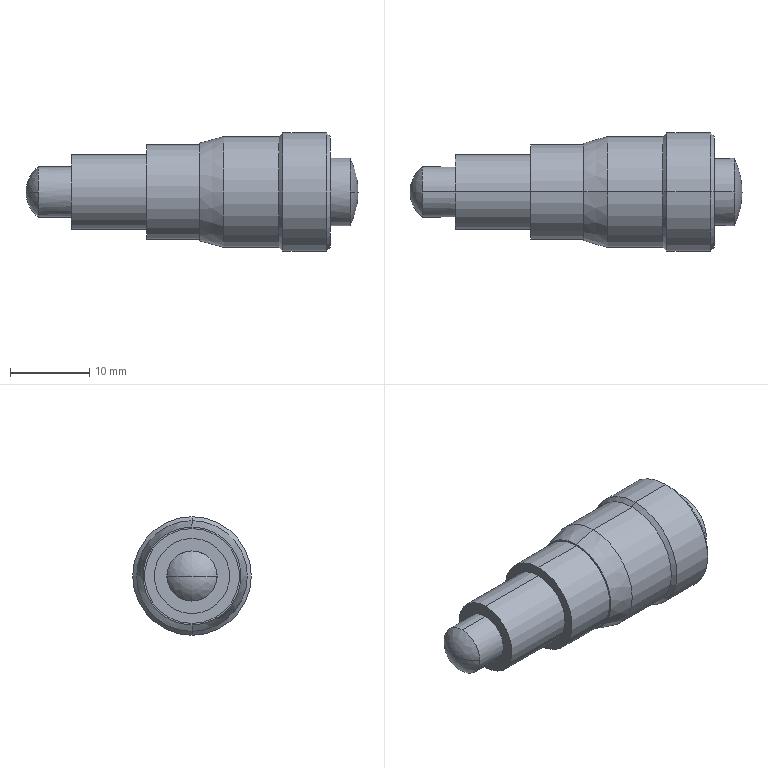Part | SolidWorks | features BaseBody 1 | 1 solid | 26 faces | box 42 x 15 x 15 mm | volume 4392 mm3 | cylinder 12 | cone 6 | spline 4 | plane 4 | commonest cylinder face diameters 6.35 x2 8.5 x2 9.5 x2 12 x2 14 x2 15 x2
STEP:
#1=CARTESIAN_POINT('',(26.75,0.,0.));
#2=VERTEX_POINT('',#1);
#3=CARTESIAN_POINT('',(25.746,4.25,0.));
#4=VERTEX_POINT('',#3);
#5=CARTESIAN_POINT('',(17.25,0.,0.));
#6=DIRECTION('',(0.,0.,1.));
#7=DIRECTION('',(1.,0.,0.));
#8=AXIS2_PLACEMENT_3D('',#5,#6,#7);
#9=CIRCLE('',#8,9.5);
#10=EDGE_CURVE('',#2,#4,#9,.T.);
#11=ORIENTED_EDGE('',*,*,#10,.F.);
#12=CARTESIAN_POINT('',(25.746,-4.25,0.));
#13=VERTEX_POINT('',#12);
#14=CARTESIAN_POINT('',(17.25,0.,0.));
#15=DIRECTION('',(0.,0.,-1.));
#16=DIRECTION('',(1.,0.,0.));
#17=AXIS2_PLACEMENT_3D('',#14,#15,#16);
#18=CIRCLE('',#17,9.5);
#19=EDGE_CURVE('',#2,#13,#18,.T.);
#20=ORIENTED_EDGE('',*,*,#19,.T.);
#21=CARTESIAN_POINT('',(25.746,0.,-4.25));
#22=VERTEX_POINT('',#21);
#23=CARTESIAN_POINT('',(25.746,0.,0.));
#24=DIRECTION('',(-1.,0.,0.));
#25=DIRECTION('',(0.,0.,-1.));
#26=AXIS2_PLACEMENT_3D('',#23,#24,#25);
#27=CIRCLE('',#26,4.25);
#28=EDGE_CURVE('',#22,#13,#27,.T.);
#29=ORIENTED_EDGE('',*,*,#28,.F.);
#30=CARTESIAN_POINT('',(25.746,0.,0.));
#31=DIRECTION('',(-1.,0.,0.));
#32=DIRECTION('',(0.,0.,-1.));
#33=AXIS2_PLACEMENT_3D('',#30,#31,#32);
#34=CIRCLE('',#33,4.25);
#35=EDGE_CURVE('',#4,#22,#34,.T.);
#36=ORIENTED_EDGE('',*,*,#35,.F.);
#37=EDGE_LOOP('',(#11,#20,#29,#36));
#38=FACE_OUTER_BOUND('',#37,.T.);
#39=CARTESIAN_POINT('',(26.75,0.,0.));
#40=CARTESIAN_POINT('',(26.75,0.,0.));
#41=CARTESIAN_POINT('',(26.75,0.,0.));
#42=CARTESIAN_POINT('',(26.75,0.,0.));
#43=CARTESIAN_POINT('',(26.75,-1.482,0.));
#44=CARTESIAN_POINT('',(26.75,-1.482,-2.964));
#45=CARTESIAN_POINT('',(26.75,1.482,-2.964));
#46=CARTESIAN_POINT('',(26.75,1.482,0.));
#47=CARTESIAN_POINT('',(26.409,-2.924,0.));
#48=CARTESIAN_POINT('',(26.409,-2.924,-5.849));
#49=CARTESIAN_POINT('',(26.409,2.924,-5.849));
#50=CARTESIAN_POINT('',(26.409,2.924,0.));
#51=CARTESIAN_POINT('',(25.746,-4.25,0.));
#52=CARTESIAN_POINT('',(25.746,-4.25,-8.5));
#53=CARTESIAN_POINT('',(25.746,4.25,-8.5));
#54=CARTESIAN_POINT('',(25.746,4.25,0.));
#55=(BOUNDED_SURFACE()B_SPLINE_SURFACE(3,3,((#39,#40,#41,#42),(#43,#44,#45,#46),(#47,#48,#49,#50),(#51,#52,#53,#54)),.UNSPECIFIED.,.F.,.F.,.T.)B_SPLINE_SURFACE_WITH_KNOTS((4,4),(4,4),(0.,1.),(0.,1.),.UNSPECIFIED.)GEOMETRIC_REPRESENTATION_ITEM()RATIONAL_B_SPLINE_SURFACE(((1.,0.3333,0.3333,1.),(0.9822,0.3274,0.3274,0.9822),(0.9822,0.3274,0.3274,0.9822),(1.,0.3333,0.3333,1.)))REPRESENTATION_ITEM('')SURFACE());
#56=ADVANCED_FACE('',(#38),#55,.T.);
#57=CARTESIAN_POINT('',(-13.683,-3.175,0.));
#58=VERTEX_POINT('',#57);
#59=CARTESIAN_POINT('',(-13.683,0.,-3.175));
#60=VERTEX_POINT('',#59);
#61=CARTESIAN_POINT('',(-13.683,0.,0.));
#62=DIRECTION('',(1.,0.,0.));
#63=DIRECTION('',(0.,0.,-1.));
#64=AXIS2_PLACEMENT_3D('',#61,#62,#63);
#65=CIRCLE('',#64,3.175);
#66=EDGE_CURVE('',#58,#60,#65,.T.);
#67=ORIENTED_EDGE('',*,*,#66,.F.);
#68=CARTESIAN_POINT('',(-15.25,0.,0.));
#69=VERTEX_POINT('',#68);
#70=CARTESIAN_POINT('',(-11.25,0.,0.));
#71=DIRECTION('',(0.,0.,-1.));
#72=DIRECTION('',(1.,0.,0.));
#73=AXIS2_PLACEMENT_3D('',#70,#71,#72);
#74=CIRCLE('',#73,4.);
#75=EDGE_CURVE('',#58,#69,#74,.T.);
#76=ORIENTED_EDGE('',*,*,#75,.T.);
#77=CARTESIAN_POINT('',(-13.683,3.175,0.));
#78=VERTEX_POINT('',#77);
#79=CARTESIAN_POINT('',(-11.25,0.,0.));
#80=DIRECTION('',(0.,0.,1.));
#81=DIRECTION('',(1.,0.,0.));
#82=AXIS2_PLACEMENT_3D('',#79,#80,#81);
#83=CIRCLE('',#82,4.);
#84=EDGE_CURVE('',#78,#69,#83,.T.);
#85=ORIENTED_EDGE('',*,*,#84,.F.);
#86=CARTESIAN_POINT('',(-13.683,0.,0.));
#87=DIRECTION('',(1.,0.,0.));
#88=DIRECTION('',(0.,0.,-1.));
#89=AXIS2_PLACEMENT_3D('',#86,#87,#88);
#90=CIRCLE('',#89,3.175);
#91=EDGE_CURVE('',#60,#78,#90,.T.);
#92=ORIENTED_EDGE('',*,*,#91,.F.);
#93=EDGE_LOOP('',(#67,#76,#85,#92));
#94=FACE_OUTER_BOUND('',#93,.T.);
#95=CARTESIAN_POINT('',(-13.683,-3.175,0.));
#96=CARTESIAN_POINT('',(-13.683,-3.175,-6.35));
#97=CARTESIAN_POINT('',(-13.683,3.175,-6.35));
#98=CARTESIAN_POINT('',(-13.683,3.175,0.));
#99=CARTESIAN_POINT('',(-14.689,-2.404,0.));
#100=CARTESIAN_POINT('',(-14.689,-2.404,-4.808));
#101=CARTESIAN_POINT('',(-14.689,2.404,-4.808));
#102=CARTESIAN_POINT('',(-14.689,2.404,0.));
#103=CARTESIAN_POINT('',(-15.25,-1.267,0.));
#104=CARTESIAN_POINT('',(-15.25,-1.267,-2.535));
#105=CARTESIAN_POINT('',(-15.25,1.267,-2.535));
#106=CARTESIAN_POINT('',(-15.25,1.267,0.));
#107=CARTESIAN_POINT('',(-15.25,0.,0.));
#108=CARTESIAN_POINT('',(-15.25,0.,0.));
#109=CARTESIAN_POINT('',(-15.25,0.,0.));
#110=CARTESIAN_POINT('',(-15.25,0.,0.));
#111=(BOUNDED_SURFACE()B_SPLINE_SURFACE(3,3,((#95,#96,#97,#98),(#99,#100,#101,#102),(#103,#104,#105,#106),(#107,#108,#109,#110)),.UNSPECIFIED.,.F.,.F.,.F.)B_SPLINE_SURFACE_WITH_KNOTS((4,4),(4,4),(0.,1.),(0.,1.),.UNSPECIFIED.)GEOMETRIC_REPRESENTATION_ITEM()RATIONAL_B_SPLINE_SURFACE(((1.,0.3333,0.3333,1.),(0.9312,0.3104,0.3104,0.9312),(0.9312,0.3104,0.3104,0.9312),(1.,0.3333,0.3333,1.)))REPRESENTATION_ITEM('')SURFACE());
#112=ADVANCED_FACE('',(#94),#111,.T.);
#113=CARTESIAN_POINT('',(9.75,0.,-7.));
#114=VERTEX_POINT('',#113);
#115=CARTESIAN_POINT('',(9.75,0.,7.));
#116=VERTEX_POINT('',#115);
#117=CARTESIAN_POINT('',(9.75,0.,0.));
#118=DIRECTION('',(1.,0.,0.));
#119=DIRECTION('',(0.,0.,-1.));
#120=AXIS2_PLACEMENT_3D('',#117,#118,#119);
#121=CIRCLE('',#120,7.);
#122=EDGE_CURVE('',#114,#116,#121,.T.);
#123=ORIENTED_EDGE('',*,*,#122,.T.);
#124=CARTESIAN_POINT('',(16.75,0.,7.));
#125=VERTEX_POINT('',#124);
#126=CARTESIAN_POINT('',(13.25,0.,7.));
#127=DIRECTION('',(1.,0.,0.));
#128=VECTOR('',#127,1000.);
#129=LINE('',#126,#128);
#130=EDGE_CURVE('',#116,#125,#129,.T.);
#131=ORIENTED_EDGE('',*,*,#130,.T.);
#132=CARTESIAN_POINT('',(16.75,0.,-7.));
#133=VERTEX_POINT('',#132);
#134=CARTESIAN_POINT('',(16.75,0.,0.));
#135=DIRECTION('',(-1.,0.,0.));
#136=DIRECTION('',(0.,0.,-1.));
#137=AXIS2_PLACEMENT_3D('',#134,#135,#136);
#138=CIRCLE('',#137,7.);
#139=EDGE_CURVE('',#125,#133,#138,.T.);
#140=ORIENTED_EDGE('',*,*,#139,.T.);
#141=CARTESIAN_POINT('',(13.25,0.,-7.));
#142=DIRECTION('',(1.,0.,0.));
#143=VECTOR('',#142,1000.);
#144=LINE('',#141,#143);
#145=EDGE_CURVE('',#114,#133,#144,.T.);
#146=ORIENTED_EDGE('',*,*,#145,.F.);
#147=EDGE_LOOP('',(#123,#131,#140,#146));
#148=FACE_OUTER_BOUND('',#147,.T.);
#149=CARTESIAN_POINT('',(13.25,0.,0.));
#150=DIRECTION('',(1.,0.,0.));
#151=DIRECTION('',(0.,0.,-1.));
#152=AXIS2_PLACEMENT_3D('',#149,#150,#151);
#153=CYLINDRICAL_SURFACE('',#152,7.);
#154=ADVANCED_FACE('',(#148),#153,.T.);
#155=CARTESIAN_POINT('',(6.75,0.,-6.196));
#156=VERTEX_POINT('',#155);
#157=CARTESIAN_POINT('',(6.75,0.,6.196));
#158=VERTEX_POINT('',#157);
#159=CARTESIAN_POINT('',(6.75,0.,0.));
#160=DIRECTION('',(1.,0.,0.));
#161=DIRECTION('',(0.,0.,-1.));
#162=AXIS2_PLACEMENT_3D('',#159,#160,#161);
#163=CIRCLE('',#162,6.196);
#164=EDGE_CURVE('',#156,#158,#163,.T.);
#165=ORIENTED_EDGE('',*,*,#164,.T.);
#166=CARTESIAN_POINT('',(9.75,0.,7.));
#167=DIRECTION('',(0.9659,0.,0.2588));
#168=VECTOR('',#167,1000.);
#169=LINE('',#166,#168);
#170=EDGE_CURVE('',#158,#116,#169,.T.);
#171=ORIENTED_EDGE('',*,*,#170,.T.);
#172=ORIENTED_EDGE('',*,*,#122,.F.);
#173=CARTESIAN_POINT('',(9.75,0.,-7.));
#174=DIRECTION('',(0.9659,0.,-0.2588));
#175=VECTOR('',#174,1000.);
#176=LINE('',#173,#175);
#177=EDGE_CURVE('',#156,#114,#176,.T.);
#178=ORIENTED_EDGE('',*,*,#177,.F.);
#179=EDGE_LOOP('',(#165,#171,#172,#178));
#180=FACE_OUTER_BOUND('',#179,.T.);
#181=CARTESIAN_POINT('',(9.75,0.,0.));
#182=DIRECTION('',(1.,0.,0.));
#183=DIRECTION('',(0.,0.,-1.));
#184=AXIS2_PLACEMENT_3D('',#181,#182,#183);
#185=CONICAL_SURFACE('',#184,7.,0.2618);
#186=ADVANCED_FACE('',(#180),#185,.T.);
#187=ORIENTED_EDGE('',*,*,#139,.F.);
#188=CARTESIAN_POINT('',(17.25,0.,7.5));
#189=VERTEX_POINT('',#188);
#190=CARTESIAN_POINT('',(17.25,0.,7.5));
#191=DIRECTION('',(0.7071,0.,0.7071));
#192=VECTOR('',#191,1000.);
#193=LINE('',#190,#192);
#194=EDGE_CURVE('',#125,#189,#193,.T.);
#195=ORIENTED_EDGE('',*,*,#194,.T.);
#196=CARTESIAN_POINT('',(17.25,0.,-7.5));
#197=VERTEX_POINT('',#196);
#198=CARTESIAN_POINT('',(17.25,0.,0.));
#199=DIRECTION('',(-1.,0.,0.));
#200=DIRECTION('',(0.,1.,0.));
#201=AXIS2_PLACEMENT_3D('',#198,#199,#200);
#202=CIRCLE('',#201,7.5);
#203=EDGE_CURVE('',#189,#197,#202,.T.);
#204=ORIENTED_EDGE('',*,*,#203,.T.);
#205=CARTESIAN_POINT('',(17.25,0.,-7.5));
#206=DIRECTION('',(0.7071,0.,-0.7071));
#207=VECTOR('',#206,1000.);
#208=LINE('',#205,#207);
#209=EDGE_CURVE('',#133,#197,#208,.T.);
#210=ORIENTED_EDGE('',*,*,#209,.F.);
#211=EDGE_LOOP('',(#187,#195,#204,#210));
#212=FACE_OUTER_BOUND('',#211,.T.);
#213=CARTESIAN_POINT('',(17.25,0.,0.));
#214=DIRECTION('',(1.,0.,0.));
#215=DIRECTION('',(0.,0.,-1.));
#216=AXIS2_PLACEMENT_3D('',#213,#214,#215);
#217=CONICAL_SURFACE('',#216,7.5,0.7854);
#218=ADVANCED_FACE('',(#212),#217,.T.);
#219=ORIENTED_EDGE('',*,*,#203,.F.);
#220=CARTESIAN_POINT('',(22.75,0.,7.5));
#221=VERTEX_POINT('',#220);
#222=CARTESIAN_POINT('',(20.,0.,7.5));
#223=DIRECTION('',(1.,0.,0.));
#224=VECTOR('',#223,1000.);
#225=LINE('',#222,#224);
#226=EDGE_CURVE('',#189,#221,#225,.T.);
#227=ORIENTED_EDGE('',*,*,#226,.T.);
#228=CARTESIAN_POINT('',(22.75,0.,-7.5));
#229=VERTEX_POINT('',#228);
#230=CARTESIAN_POINT('',(22.75,0.,0.));
#231=DIRECTION('',(-1.,0.,0.));
#232=DIRECTION('',(0.,0.,-1.));
#233=AXIS2_PLACEMENT_3D('',#230,#231,#232);
#234=CIRCLE('',#233,7.5);
#235=EDGE_CURVE('',#221,#229,#234,.T.);
#236=ORIENTED_EDGE('',*,*,#235,.T.);
#237=CARTESIAN_POINT('',(20.,0.,-7.5));
#238=DIRECTION('',(1.,0.,0.));
#239=VECTOR('',#238,1000.);
#240=LINE('',#237,#239);
#241=EDGE_CURVE('',#197,#229,#240,.T.);
#242=ORIENTED_EDGE('',*,*,#241,.F.);
#243=EDGE_LOOP('',(#219,#227,#236,#242));
#244=FACE_OUTER_BOUND('',#243,.T.);
#245=CARTESIAN_POINT('',(20.,0.,0.));
#246=DIRECTION('',(1.,0.,0.));
#247=DIRECTION('',(0.,0.,-1.));
#248=AXIS2_PLACEMENT_3D('',#245,#246,#247);
#249=CYLINDRICAL_SURFACE('',#248,7.5);
#250=ADVANCED_FACE('',(#244),#249,.T.);
#251=CARTESIAN_POINT('',(0.,0.,-6.));
#252=VERTEX_POINT('',#251);
#253=CARTESIAN_POINT('',(0.,0.,6.));
#254=VERTEX_POINT('',#253);
#255=CARTESIAN_POINT('',(0.,0.,0.));
#256=DIRECTION('',(1.,0.,0.));
#257=DIRECTION('',(0.,0.,-1.));
#258=AXIS2_PLACEMENT_3D('',#255,#256,#257);
#259=CIRCLE('',#258,6.);
#260=EDGE_CURVE('',#252,#254,#259,.T.);
#261=ORIENTED_EDGE('',*,*,#260,.T.);
#262=CARTESIAN_POINT('',(6.75,0.,6.));
#263=VERTEX_POINT('',#262);
#264=CARTESIAN_POINT('',(3.375,0.,6.));
#265=DIRECTION('',(1.,0.,0.));
#266=VECTOR('',#265,1000.);
#267=LINE('',#264,#266);
#268=EDGE_CURVE('',#254,#263,#267,.T.);
#269=ORIENTED_EDGE('',*,*,#268,.T.);
#270=CARTESIAN_POINT('',(6.75,0.,-6.));
#271=VERTEX_POINT('',#270);
#272=CARTESIAN_POINT('',(6.75,0.,0.));
#273=DIRECTION('',(1.,0.,0.));
#274=DIRECTION('',(0.,0.,-1.));
#275=AXIS2_PLACEMENT_3D('',#272,#273,#274);
#276=CIRCLE('',#275,6.);
#277=EDGE_CURVE('',#271,#263,#276,.T.);
#278=ORIENTED_EDGE('',*,*,#277,.F.);
#279=CARTESIAN_POINT('',(3.375,0.,-6.));
#280=DIRECTION('',(1.,0.,0.));
#281=VECTOR('',#280,1000.);
#282=LINE('',#279,#281);
#283=EDGE_CURVE('',#252,#271,#282,.T.);
#284=ORIENTED_EDGE('',*,*,#283,.F.);
#285=EDGE_LOOP('',(#261,#269,#278,#284));
#286=FACE_OUTER_BOUND('',#285,.T.);
#287=CARTESIAN_POINT('',(3.375,0.,0.));
#288=DIRECTION('',(1.,0.,0.));
#289=DIRECTION('',(0.,0.,-1.));
#290=AXIS2_PLACEMENT_3D('',#287,#288,#289);
#291=CYLINDRICAL_SURFACE('',#290,6.);
#292=ADVANCED_FACE('',(#286),#291,.T.);
#293=CARTESIAN_POINT('',(23.25,0.,7.));
#294=VERTEX_POINT('',#293);
#295=CARTESIAN_POINT('',(23.25,0.,-7.));
#296=VERTEX_POINT('',#295);
#297=CARTESIAN_POINT('',(23.25,0.,0.));
#298=DIRECTION('',(-1.,0.,0.));
#299=DIRECTION('',(0.,0.,1.));
#300=AXIS2_PLACEMENT_3D('',#297,#298,#299);
#301=CIRCLE('',#300,7.);
#302=EDGE_CURVE('',#294,#296,#301,.T.);
#303=ORIENTED_EDGE('',*,*,#302,.T.);
#304=CARTESIAN_POINT('',(22.75,0.,-7.5));
#305=DIRECTION('',(-0.7071,0.,-0.7071));
#306=VECTOR('',#305,1000.);
#307=LINE('',#304,#306);
#308=EDGE_CURVE('',#296,#229,#307,.T.);
#309=ORIENTED_EDGE('',*,*,#308,.T.);
#310=ORIENTED_EDGE('',*,*,#235,.F.);
#311=CARTESIAN_POINT('',(22.75,0.,7.5));
#312=DIRECTION('',(-0.7071,0.,0.7071));
#313=VECTOR('',#312,1000.);
#314=LINE('',#311,#313);
#315=EDGE_CURVE('',#294,#221,#314,.T.);
#316=ORIENTED_EDGE('',*,*,#315,.F.);
#317=EDGE_LOOP('',(#303,#309,#310,#316));
#318=FACE_OUTER_BOUND('',#317,.T.);
#319=CARTESIAN_POINT('',(22.75,0.,0.));
#320=DIRECTION('',(-1.,0.,0.));
#321=DIRECTION('',(0.,0.,1.));
#322=AXIS2_PLACEMENT_3D('',#319,#320,#321);
#323=CONICAL_SURFACE('',#322,7.5,0.7854);
#324=ADVANCED_FACE('',(#318),#323,.T.);
#325=CARTESIAN_POINT('',(-9.5,0.,-4.75));
#326=VERTEX_POINT('',#325);
#327=CARTESIAN_POINT('',(-9.5,0.,4.75));
#328=VERTEX_POINT('',#327);
#329=CARTESIAN_POINT('',(-9.5,0.,0.));
#330=DIRECTION('',(1.,0.,0.));
#331=DIRECTION('',(0.,0.,-1.));
#332=AXIS2_PLACEMENT_3D('',#329,#330,#331);
#333=CIRCLE('',#332,4.75);
#334=EDGE_CURVE('',#326,#328,#333,.T.);
#335=ORIENTED_EDGE('',*,*,#334,.T.);
#336=CARTESIAN_POINT('',(0.,0.,4.75));
#337=VERTEX_POINT('',#336);
#338=CARTESIAN_POINT('',(-4.75,0.,4.75));
#339=DIRECTION('',(1.,0.,0.));
#340=VECTOR('',#339,1000.);
#341=LINE('',#338,#340);
#342=EDGE_CURVE('',#328,#337,#341,.T.);
#343=ORIENTED_EDGE('',*,*,#342,.T.);
#344=CARTESIAN_POINT('',(0.,0.,-4.75));
#345=VERTEX_POINT('',#344);
#346=CARTESIAN_POINT('',(0.,0.,0.));
#347=DIRECTION('',(1.,0.,0.));
#348=DIRECTION('',(0.,0.,-1.));
#349=AXIS2_PLACEMENT_3D('',#346,#347,#348);
#350=CIRCLE('',#349,4.75);
#351=EDGE_CURVE('',#345,#337,#350,.T.);
#352=ORIENTED_EDGE('',*,*,#351,.F.);
#353=CARTESIAN_POINT('',(-4.75,0.,-4.75));
#354=DIRECTION('',(1.,0.,0.));
#355=VECTOR('',#354,1000.);
#356=LINE('',#353,#355);
#357=EDGE_CURVE('',#326,#345,#356,.T.);
#358=ORIENTED_EDGE('',*,*,#357,.F.);
#359=EDGE_LOOP('',(#335,#343,#352,#358));
#360=FACE_OUTER_BOUND('',#359,.T.);
#361=CARTESIAN_POINT('',(-4.75,0.,0.));
#362=DIRECTION('',(1.,0.,0.));
#363=DIRECTION('',(0.,0.,-1.));
#364=AXIS2_PLACEMENT_3D('',#361,#362,#363);
#365=CYLINDRICAL_SURFACE('',#364,4.75);
#366=ADVANCED_FACE('',(#360),#365,.T.);
#367=CARTESIAN_POINT('',(23.25,0.,4.25));
#368=VERTEX_POINT('',#367);
#369=CARTESIAN_POINT('',(23.25,0.,-4.25));
#370=VERTEX_POINT('',#369);
#371=CARTESIAN_POINT('',(23.25,0.,0.));
#372=DIRECTION('',(-1.,0.,0.));
#373=DIRECTION('',(0.,0.,-1.));
#374=AXIS2_PLACEMENT_3D('',#371,#372,#373);
#375=CIRCLE('',#374,4.25);
#376=EDGE_CURVE('',#368,#370,#375,.T.);
#377=ORIENTED_EDGE('',*,*,#376,.F.);
#378=CARTESIAN_POINT('',(25.746,0.,4.25));
#379=VERTEX_POINT('',#378);
#380=CARTESIAN_POINT('',(24.498,0.,4.25));
#381=DIRECTION('',(1.,0.,0.));
#382=VECTOR('',#381,1000.);
#383=LINE('',#380,#382);
#384=EDGE_CURVE('',#368,#379,#383,.T.);
#385=ORIENTED_EDGE('',*,*,#384,.T.);
#386=CARTESIAN_POINT('',(25.746,0.,0.));
#387=DIRECTION('',(-1.,0.,0.));
#388=DIRECTION('',(0.,0.,-1.));
#389=AXIS2_PLACEMENT_3D('',#386,#387,#388);
#390=CIRCLE('',#389,4.25);
#391=EDGE_CURVE('',#379,#4,#390,.T.);
#392=ORIENTED_EDGE('',*,*,#391,.T.);
#393=ORIENTED_EDGE('',*,*,#35,.T.);
#394=CARTESIAN_POINT('',(24.498,0.,-4.25));
#395=DIRECTION('',(1.,0.,0.));
#396=VECTOR('',#395,1000.);
#397=LINE('',#394,#396);
#398=EDGE_CURVE('',#370,#22,#397,.T.);
#399=ORIENTED_EDGE('',*,*,#398,.F.);
#400=EDGE_LOOP('',(#377,#385,#392,#393,#399));
#401=FACE_OUTER_BOUND('',#400,.T.);
#402=CARTESIAN_POINT('',(24.498,0.,0.));
#403=DIRECTION('',(1.,0.,0.));
#404=DIRECTION('',(0.,0.,-1.));
#405=AXIS2_PLACEMENT_3D('',#402,#403,#404);
#406=CYLINDRICAL_SURFACE('',#405,4.25);
#407=ADVANCED_FACE('',(#401),#406,.T.);
#408=ORIENTED_EDGE('',*,*,#91,.T.);
#409=CARTESIAN_POINT('',(-13.683,0.,3.175));
#410=VERTEX_POINT('',#409);
#411=CARTESIAN_POINT('',(-13.683,0.,0.));
#412=DIRECTION('',(1.,0.,0.));
#413=DIRECTION('',(0.,0.,-1.));
#414=AXIS2_PLACEMENT_3D('',#411,#412,#413);
#415=CIRCLE('',#414,3.175);
#416=EDGE_CURVE('',#78,#410,#415,.T.);
#417=ORIENTED_EDGE('',*,*,#416,.T.);
#418=CARTESIAN_POINT('',(-9.5,0.,3.175));
#419=VERTEX_POINT('',#418);
#420=CARTESIAN_POINT('',(-11.591,0.,3.175));
#421=DIRECTION('',(1.,0.,0.));
#422=VECTOR('',#421,1000.);
#423=LINE('',#420,#422);
#424=EDGE_CURVE('',#410,#419,#423,.T.);
#425=ORIENTED_EDGE('',*,*,#424,.T.);
#426=CARTESIAN_POINT('',(-9.5,0.,-3.175));
#427=VERTEX_POINT('',#426);
#428=CARTESIAN_POINT('',(-9.5,0.,0.));
#429=DIRECTION('',(1.,0.,0.));
#430=DIRECTION('',(0.,0.,-1.));
#431=AXIS2_PLACEMENT_3D('',#428,#429,#430);
#432=CIRCLE('',#431,3.175);
#433=EDGE_CURVE('',#427,#419,#432,.T.);
#434=ORIENTED_EDGE('',*,*,#433,.F.);
#435=CARTESIAN_POINT('',(-11.591,0.,-3.175));
#436=DIRECTION('',(1.,0.,0.));
#437=VECTOR('',#436,1000.);
#438=LINE('',#435,#437);
#439=EDGE_CURVE('',#60,#427,#438,.T.);
#440=ORIENTED_EDGE('',*,*,#439,.F.);
#441=EDGE_LOOP('',(#408,#417,#425,#434,#440));
#442=FACE_OUTER_BOUND('',#441,.T.);
#443=CARTESIAN_POINT('',(-11.591,0.,0.));
#444=DIRECTION('',(1.,0.,0.));
#445=DIRECTION('',(0.,0.,-1.));
#446=AXIS2_PLACEMENT_3D('',#443,#444,#445);
#447=CYLINDRICAL_SURFACE('',#446,3.175);
#448=ADVANCED_FACE('',(#442),#447,.T.);
#449=ORIENTED_EDGE('',*,*,#130,.F.);
#450=CARTESIAN_POINT('',(9.75,0.,0.));
#451=DIRECTION('',(1.,0.,0.));
#452=DIRECTION('',(0.,0.,-1.));
#453=AXIS2_PLACEMENT_3D('',#450,#451,#452);
#454=CIRCLE('',#453,7.);
#455=EDGE_CURVE('',#116,#114,#454,.T.);
#456=ORIENTED_EDGE('',*,*,#455,.T.);
#457=ORIENTED_EDGE('',*,*,#145,.T.);
#458=CARTESIAN_POINT('',(16.75,0.,0.));
#459=DIRECTION('',(-1.,0.,0.));
#460=DIRECTION('',(0.,0.,-1.));
#461=AXIS2_PLACEMENT_3D('',#458,#459,#460);
#462=CIRCLE('',#461,7.);
#463=EDGE_CURVE('',#133,#125,#462,.T.);
#464=ORIENTED_EDGE('',*,*,#463,.T.);
#465=EDGE_LOOP('',(#449,#456,#457,#464));
#466=FACE_OUTER_BOUND('',#465,.T.);
#467=CARTESIAN_POINT('',(13.25,0.,0.));
#468=DIRECTION('',(1.,0.,0.));
#469=DIRECTION('',(0.,0.,-1.));
#470=AXIS2_PLACEMENT_3D('',#467,#468,#469);
#471=CYLINDRICAL_SURFACE('',#470,7.);
#472=ADVANCED_FACE('',(#466),#471,.T.);
#473=ORIENTED_EDGE('',*,*,#170,.F.);
#474=CARTESIAN_POINT('',(6.75,0.,0.));
#475=DIRECTION('',(1.,0.,0.));
#476=DIRECTION('',(0.,0.,-1.));
#477=AXIS2_PLACEMENT_3D('',#474,#475,#476);
#478=CIRCLE('',#477,6.196);
#479=EDGE_CURVE('',#158,#156,#478,.T.);
#480=ORIENTED_EDGE('',*,*,#479,.T.);
#481=ORIENTED_EDGE('',*,*,#177,.T.);
#482=ORIENTED_EDGE('',*,*,#455,.F.);
#483=EDGE_LOOP('',(#473,#480,#481,#482));
#484=FACE_OUTER_BOUND('',#483,.T.);
#485=CARTESIAN_POINT('',(9.75,0.,0.));
#486=DIRECTION('',(1.,0.,0.));
#487=DIRECTION('',(0.,0.,-1.));
#488=AXIS2_PLACEMENT_3D('',#485,#486,#487);
#489=CONICAL_SURFACE('',#488,7.,0.2618);
#490=ADVANCED_FACE('',(#484),#489,.T.);
#491=ORIENTED_EDGE('',*,*,#194,.F.);
#492=ORIENTED_EDGE('',*,*,#463,.F.);
#493=ORIENTED_EDGE('',*,*,#209,.T.);
#494=CARTESIAN_POINT('',(17.25,0.,0.));
#495=DIRECTION('',(-1.,0.,0.));
#496=DIRECTION('',(0.,1.,0.));
#497=AXIS2_PLACEMENT_3D('',#494,#495,#496);
#498=CIRCLE('',#497,7.5);
#499=EDGE_CURVE('',#197,#189,#498,.T.);
#500=ORIENTED_EDGE('',*,*,#499,.T.);
#501=EDGE_LOOP('',(#491,#492,#493,#500));
#502=FACE_OUTER_BOUND('',#501,.T.);
#503=CARTESIAN_POINT('',(17.25,0.,0.));
#504=DIRECTION('',(1.,0.,0.));
#505=DIRECTION('',(0.,0.,-1.));
#506=AXIS2_PLACEMENT_3D('',#503,#504,#505);
#507=CONICAL_SURFACE('',#506,7.5,0.7854);
#508=ADVANCED_FACE('',(#502),#507,.T.);
#509=ORIENTED_EDGE('',*,*,#164,.F.);
#510=ORIENTED_EDGE('',*,*,#479,.F.);
#511=EDGE_LOOP('',(#509,#510));
#512=FACE_OUTER_BOUND('',#511,.T.);
#513=ORIENTED_EDGE('',*,*,#277,.T.);
#514=CARTESIAN_POINT('',(6.75,0.,0.));
#515=DIRECTION('',(1.,0.,0.));
#516=DIRECTION('',(0.,0.,-1.));
#517=AXIS2_PLACEMENT_3D('',#514,#515,#516);
#518=CIRCLE('',#517,6.);
#519=EDGE_CURVE('',#263,#271,#518,.T.);
#520=ORIENTED_EDGE('',*,*,#519,.T.);
#521=EDGE_LOOP('',(#513,#520));
#522=FACE_BOUND('',#521,.T.);
#523=CARTESIAN_POINT('',(6.75,6.098,0.));
#524=DIRECTION('',(-1.,0.,0.));
#525=DIRECTION('',(0.,0.,1.));
#526=AXIS2_PLACEMENT_3D('',#523,#524,#525);
#527=PLANE('',#526);
#528=ADVANCED_FACE('',(#512,#522),#527,.T.);
#529=ORIENTED_EDGE('',*,*,#226,.F.);
#530=ORIENTED_EDGE('',*,*,#499,.F.);
#531=ORIENTED_EDGE('',*,*,#241,.T.);
#532=CARTESIAN_POINT('',(22.75,0.,0.));
#533=DIRECTION('',(-1.,0.,0.));
#534=DIRECTION('',(0.,0.,-1.));
#535=AXIS2_PLACEMENT_3D('',#532,#533,#534);
#536=CIRCLE('',#535,7.5);
#537=EDGE_CURVE('',#229,#221,#536,.T.);
#538=ORIENTED_EDGE('',*,*,#537,.T.);
#539=EDGE_LOOP('',(#529,#530,#531,#538));
#540=FACE_OUTER_BOUND('',#539,.T.);
#541=CARTESIAN_POINT('',(20.,0.,0.));
#542=DIRECTION('',(1.,0.,0.));
#543=DIRECTION('',(0.,0.,-1.));
#544=AXIS2_PLACEMENT_3D('',#541,#542,#543);
#545=CYLINDRICAL_SURFACE('',#544,7.5);
#546=ADVANCED_FACE('',(#540),#545,.T.);
#547=ORIENTED_EDGE('',*,*,#268,.F.);
#548=CARTESIAN_POINT('',(0.,0.,0.));
#549=DIRECTION('',(1.,0.,0.));
#550=DIRECTION('',(0.,0.,-1.));
#551=AXIS2_PLACEMENT_3D('',#548,#549,#550);
#552=CIRCLE('',#551,6.);
#553=EDGE_CURVE('',#254,#252,#552,.T.);
#554=ORIENTED_EDGE('',*,*,#553,.T.);
#555=ORIENTED_EDGE('',*,*,#283,.T.);
#556=ORIENTED_EDGE('',*,*,#519,.F.);
#557=EDGE_LOOP('',(#547,#554,#555,#556));
#558=FACE_OUTER_BOUND('',#557,.T.);
#559=CARTESIAN_POINT('',(3.375,0.,0.));
#560=DIRECTION('',(1.,0.,0.));
#561=DIRECTION('',(0.,0.,-1.));
#562=AXIS2_PLACEMENT_3D('',#559,#560,#561);
#563=CYLINDRICAL_SURFACE('',#562,6.);
#564=ADVANCED_FACE('',(#558),#563,.T.);
#565=ORIENTED_EDGE('',*,*,#308,.F.);
#566=CARTESIAN_POINT('',(23.25,0.,0.));
#567=DIRECTION('',(-1.,0.,0.));
#568=DIRECTION('',(0.,0.,1.));
#569=AXIS2_PLACEMENT_3D('',#566,#567,#568);
#570=CIRCLE('',#569,7.);
#571=EDGE_CURVE('',#296,#294,#570,.T.);
#572=ORIENTED_EDGE('',*,*,#571,.T.);
#573=ORIENTED_EDGE('',*,*,#315,.T.);
#574=ORIENTED_EDGE('',*,*,#537,.F.);
#575=EDGE_LOOP('',(#565,#572,#573,#574));
#576=FACE_OUTER_BOUND('',#575,.T.);
#577=CARTESIAN_POINT('',(22.75,0.,0.));
#578=DIRECTION('',(-1.,0.,0.));
#579=DIRECTION('',(0.,0.,1.));
#580=AXIS2_PLACEMENT_3D('',#577,#578,#579);
#581=CONICAL_SURFACE('',#580,7.5,0.7854);
#582=ADVANCED_FACE('',(#576),#581,.T.);
#583=ORIENTED_EDGE('',*,*,#260,.F.);
#584=ORIENTED_EDGE('',*,*,#553,.F.);
#585=EDGE_LOOP('',(#583,#584));
#586=FACE_OUTER_BOUND('',#585,.T.);
#587=ORIENTED_EDGE('',*,*,#351,.T.);
#588=CARTESIAN_POINT('',(0.,0.,0.));
#589=DIRECTION('',(1.,0.,0.));
#590=DIRECTION('',(0.,0.,-1.));
#591=AXIS2_PLACEMENT_3D('',#588,#589,#590);
#592=CIRCLE('',#591,4.75);
#593=EDGE_CURVE('',#337,#345,#592,.T.);
#594=ORIENTED_EDGE('',*,*,#593,.T.);
#595=EDGE_LOOP('',(#587,#594));
#596=FACE_BOUND('',#595,.T.);
#597=CARTESIAN_POINT('',(0.,5.375,0.));
#598=DIRECTION('',(-1.,0.,0.));
#599=DIRECTION('',(0.,0.,1.));
#600=AXIS2_PLACEMENT_3D('',#597,#598,#599);
#601=PLANE('',#600);
#602=ADVANCED_FACE('',(#586,#596),#601,.T.);
#603=CARTESIAN_POINT('',(23.25,0.,0.));
#604=DIRECTION('',(-1.,0.,0.));
#605=DIRECTION('',(0.,0.,-1.));
#606=AXIS2_PLACEMENT_3D('',#603,#604,#605);
#607=CIRCLE('',#606,4.25);
#608=EDGE_CURVE('',#370,#368,#607,.T.);
#609=ORIENTED_EDGE('',*,*,#608,.T.);
#610=ORIENTED_EDGE('',*,*,#376,.T.);
#611=EDGE_LOOP('',(#609,#610));
#612=FACE_BOUND('',#611,.T.);
#613=ORIENTED_EDGE('',*,*,#302,.F.);
#614=ORIENTED_EDGE('',*,*,#571,.F.);
#615=EDGE_LOOP('',(#613,#614));
#616=FACE_OUTER_BOUND('',#615,.T.);
#617=CARTESIAN_POINT('',(23.25,5.625,0.));
#618=DIRECTION('',(1.,0.,0.));
#619=DIRECTION('',(0.,0.,-1.));
#620=AXIS2_PLACEMENT_3D('',#617,#618,#619);
#621=PLANE('',#620);
#622=ADVANCED_FACE('',(#612,#616),#621,.T.);
#623=ORIENTED_EDGE('',*,*,#342,.F.);
#624=CARTESIAN_POINT('',(-9.5,0.,0.));
#625=DIRECTION('',(1.,0.,0.));
#626=DIRECTION('',(0.,0.,-1.));
#627=AXIS2_PLACEMENT_3D('',#624,#625,#626);
#628=CIRCLE('',#627,4.75);
#629=EDGE_CURVE('',#328,#326,#628,.T.);
#630=ORIENTED_EDGE('',*,*,#629,.T.);
#631=ORIENTED_EDGE('',*,*,#357,.T.);
#632=ORIENTED_EDGE('',*,*,#593,.F.);
#633=EDGE_LOOP('',(#623,#630,#631,#632));
#634=FACE_OUTER_BOUND('',#633,.T.);
#635=CARTESIAN_POINT('',(-4.75,0.,0.));
#636=DIRECTION('',(1.,0.,0.));
#637=DIRECTION('',(0.,0.,-1.));
#638=AXIS2_PLACEMENT_3D('',#635,#636,#637);
#639=CYLINDRICAL_SURFACE('',#638,4.75);
#640=ADVANCED_FACE('',(#634),#639,.T.);
#641=ORIENTED_EDGE('',*,*,#384,.F.);
#642=ORIENTED_EDGE('',*,*,#608,.F.);
#643=ORIENTED_EDGE('',*,*,#398,.T.);
#644=ORIENTED_EDGE('',*,*,#28,.T.);
#645=CARTESIAN_POINT('',(25.746,0.,0.));
#646=DIRECTION('',(-1.,0.,0.));
#647=DIRECTION('',(0.,0.,-1.));
#648=AXIS2_PLACEMENT_3D('',#645,#646,#647);
#649=CIRCLE('',#648,4.25);
#650=EDGE_CURVE('',#13,#379,#649,.T.);
#651=ORIENTED_EDGE('',*,*,#650,.T.);
#652=EDGE_LOOP('',(#641,#642,#643,#644,#651));
#653=FACE_OUTER_BOUND('',#652,.T.);
#654=CARTESIAN_POINT('',(24.498,0.,0.));
#655=DIRECTION('',(1.,0.,0.));
#656=DIRECTION('',(0.,0.,-1.));
#657=AXIS2_PLACEMENT_3D('',#654,#655,#656);
#658=CYLINDRICAL_SURFACE('',#657,4.25);
#659=ADVANCED_FACE('',(#653),#658,.T.);
#660=ORIENTED_EDGE('',*,*,#334,.F.);
#661=ORIENTED_EDGE('',*,*,#629,.F.);
#662=EDGE_LOOP('',(#660,#661));
#663=FACE_OUTER_BOUND('',#662,.T.);
#664=ORIENTED_EDGE('',*,*,#433,.T.);
#665=CARTESIAN_POINT('',(-9.5,0.,0.));
#666=DIRECTION('',(1.,0.,0.));
#667=DIRECTION('',(0.,0.,-1.));
#668=AXIS2_PLACEMENT_3D('',#665,#666,#667);
#669=CIRCLE('',#668,3.175);
#670=EDGE_CURVE('',#419,#427,#669,.T.);
#671=ORIENTED_EDGE('',*,*,#670,.T.);
#672=EDGE_LOOP('',(#664,#671));
#673=FACE_BOUND('',#672,.T.);
#674=CARTESIAN_POINT('',(-9.5,3.962,0.));
#675=DIRECTION('',(-1.,0.,0.));
#676=DIRECTION('',(0.,0.,1.));
#677=AXIS2_PLACEMENT_3D('',#674,#675,#676);
#678=PLANE('',#677);
#679=ADVANCED_FACE('',(#663,#673),#678,.T.);
#680=ORIENTED_EDGE('',*,*,#19,.F.);
#681=ORIENTED_EDGE('',*,*,#10,.T.);
#682=ORIENTED_EDGE('',*,*,#391,.F.);
#683=ORIENTED_EDGE('',*,*,#650,.F.);
#684=EDGE_LOOP('',(#680,#681,#682,#683));
#685=FACE_OUTER_BOUND('',#684,.T.);
#686=CARTESIAN_POINT('',(26.75,0.,0.));
#687=CARTESIAN_POINT('',(26.75,0.,0.));
#688=CARTESIAN_POINT('',(26.75,0.,0.));
#689=CARTESIAN_POINT('',(26.75,0.,0.));
#690=CARTESIAN_POINT('',(26.75,1.482,0.));
#691=CARTESIAN_POINT('',(26.75,1.482,2.964));
#692=CARTESIAN_POINT('',(26.75,-1.482,2.964));
#693=CARTESIAN_POINT('',(26.75,-1.482,0.));
#694=CARTESIAN_POINT('',(26.409,2.924,0.));
#695=CARTESIAN_POINT('',(26.409,2.924,5.849));
#696=CARTESIAN_POINT('',(26.409,-2.924,5.849));
#697=CARTESIAN_POINT('',(26.409,-2.924,0.));
#698=CARTESIAN_POINT('',(25.746,4.25,0.));
#699=CARTESIAN_POINT('',(25.746,4.25,8.5));
#700=CARTESIAN_POINT('',(25.746,-4.25,8.5));
#701=CARTESIAN_POINT('',(25.746,-4.25,0.));
#702=(BOUNDED_SURFACE()B_SPLINE_SURFACE(3,3,((#686,#687,#688,#689),(#690,#691,#692,#693),(#694,#695,#696,#697),(#698,#699,#700,#701)),.UNSPECIFIED.,.F.,.F.,.T.)B_SPLINE_SURFACE_WITH_KNOTS((4,4),(4,4),(0.,1.),(0.,1.),.UNSPECIFIED.)GEOMETRIC_REPRESENTATION_ITEM()RATIONAL_B_SPLINE_SURFACE(((1.,0.3333,0.3333,1.),(0.9822,0.3274,0.3274,0.9822),(0.9822,0.3274,0.3274,0.9822),(1.,0.3333,0.3333,1.)))REPRESENTATION_ITEM('')SURFACE());
#703=ADVANCED_FACE('',(#685),#702,.T.);
#704=ORIENTED_EDGE('',*,*,#424,.F.);
#705=CARTESIAN_POINT('',(-13.683,0.,0.));
#706=DIRECTION('',(1.,0.,0.));
#707=DIRECTION('',(0.,0.,-1.));
#708=AXIS2_PLACEMENT_3D('',#705,#706,#707);
#709=CIRCLE('',#708,3.175);
#710=EDGE_CURVE('',#410,#58,#709,.T.);
#711=ORIENTED_EDGE('',*,*,#710,.T.);
#712=ORIENTED_EDGE('',*,*,#66,.T.);
#713=ORIENTED_EDGE('',*,*,#439,.T.);
#714=ORIENTED_EDGE('',*,*,#670,.F.);
#715=EDGE_LOOP('',(#704,#711,#712,#713,#714));
#716=FACE_OUTER_BOUND('',#715,.T.);
#717=CARTESIAN_POINT('',(-11.591,0.,0.));
#718=DIRECTION('',(1.,0.,0.));
#719=DIRECTION('',(0.,0.,-1.));
#720=AXIS2_PLACEMENT_3D('',#717,#718,#719);
#721=CYLINDRICAL_SURFACE('',#720,3.175);
#722=ADVANCED_FACE('',(#716),#721,.T.);
#723=ORIENTED_EDGE('',*,*,#75,.F.);
#724=ORIENTED_EDGE('',*,*,#710,.F.);
#725=ORIENTED_EDGE('',*,*,#416,.F.);
#726=ORIENTED_EDGE('',*,*,#84,.T.);
#727=EDGE_LOOP('',(#723,#724,#725,#726));
#728=FACE_OUTER_BOUND('',#727,.T.);
#729=CARTESIAN_POINT('',(-13.683,3.175,0.));
#730=CARTESIAN_POINT('',(-13.683,3.175,6.35));
#731=CARTESIAN_POINT('',(-13.683,-3.175,6.35));
#732=CARTESIAN_POINT('',(-13.683,-3.175,0.));
#733=CARTESIAN_POINT('',(-14.689,2.404,0.));
#734=CARTESIAN_POINT('',(-14.689,2.404,4.808));
#735=CARTESIAN_POINT('',(-14.689,-2.404,4.808));
#736=CARTESIAN_POINT('',(-14.689,-2.404,0.));
#737=CARTESIAN_POINT('',(-15.25,1.267,0.));
#738=CARTESIAN_POINT('',(-15.25,1.267,2.535));
#739=CARTESIAN_POINT('',(-15.25,-1.267,2.535));
#740=CARTESIAN_POINT('',(-15.25,-1.267,0.));
#741=CARTESIAN_POINT('',(-15.25,0.,0.));
#742=CARTESIAN_POINT('',(-15.25,0.,0.));
#743=CARTESIAN_POINT('',(-15.25,0.,0.));
#744=CARTESIAN_POINT('',(-15.25,0.,0.));
#745=(BOUNDED_SURFACE()B_SPLINE_SURFACE(3,3,((#729,#730,#731,#732),(#733,#734,#735,#736),(#737,#738,#739,#740),(#741,#742,#743,#744)),.UNSPECIFIED.,.F.,.F.,.F.)B_SPLINE_SURFACE_WITH_KNOTS((4,4),(4,4),(0.,1.),(0.,1.),.UNSPECIFIED.)GEOMETRIC_REPRESENTATION_ITEM()RATIONAL_B_SPLINE_SURFACE(((1.,0.3333,0.3333,1.),(0.9312,0.3104,0.3104,0.9312),(0.9312,0.3104,0.3104,0.9312),(1.,0.3333,0.3333,1.)))REPRESENTATION_ITEM('')SURFACE());
#746=ADVANCED_FACE('',(#728),#745,.T.);
#747=CLOSED_SHELL('',(#56,#112,#154,#186,#218,#250,#292,#324,#366,#407,#448,#472,#490,#508,#528,#546,#564,#582,#602,#622,#640,#659,#679,#703,#722,#746));
#748=MANIFOLD_SOLID_BREP('',#747);
#749=CARTESIAN_POINT('',(0.,0.,0.));
#750=DIRECTION('',(0.,0.,1.));
#751=DIRECTION('',(1.,0.,0.));
#752=AXIS2_PLACEMENT_3D('',#749,#750,#751);
#753=(LENGTH_UNIT()NAMED_UNIT(*)SI_UNIT(.MILLI.,.METRE.));
#754=UNCERTAINTY_MEASURE_WITH_UNIT(LENGTH_MEASURE(0.00001),#753,'','');
#755=(NAMED_UNIT(*)PLANE_ANGLE_UNIT()SI_UNIT($,.RADIAN.));
#756=(NAMED_UNIT(*)SI_UNIT($,.STERADIAN.)SOLID_ANGLE_UNIT());
#757=(GEOMETRIC_REPRESENTATION_CONTEXT(3)GLOBAL_UNCERTAINTY_ASSIGNED_CONTEXT((#754))GLOBAL_UNIT_ASSIGNED_CONTEXT((#753,#755,#756))REPRESENTATION_CONTEXT('',''));
#758=ADVANCED_BREP_SHAPE_REPRESENTATION('',(#748,#752),#757);